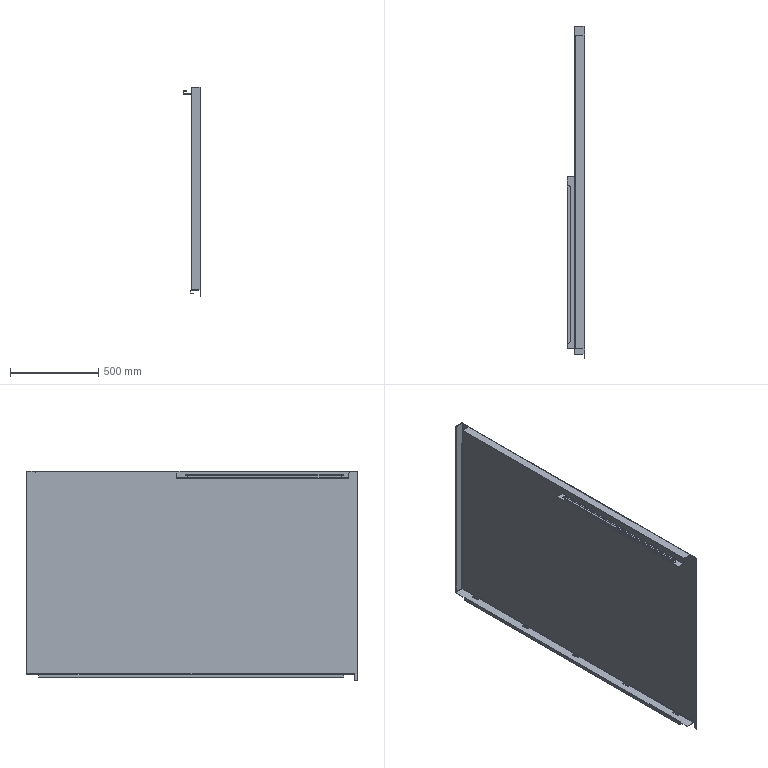Part | SolidWorks | features BaseBody 1 | 1 solid | 213 faces | box 97 x 1878 x 1185 mm | volume 5116478 mm3 | plane 189 | cylinder 20 | torus 4 | commonest cylinder face diameters 2 x9 6 x9 30 x2